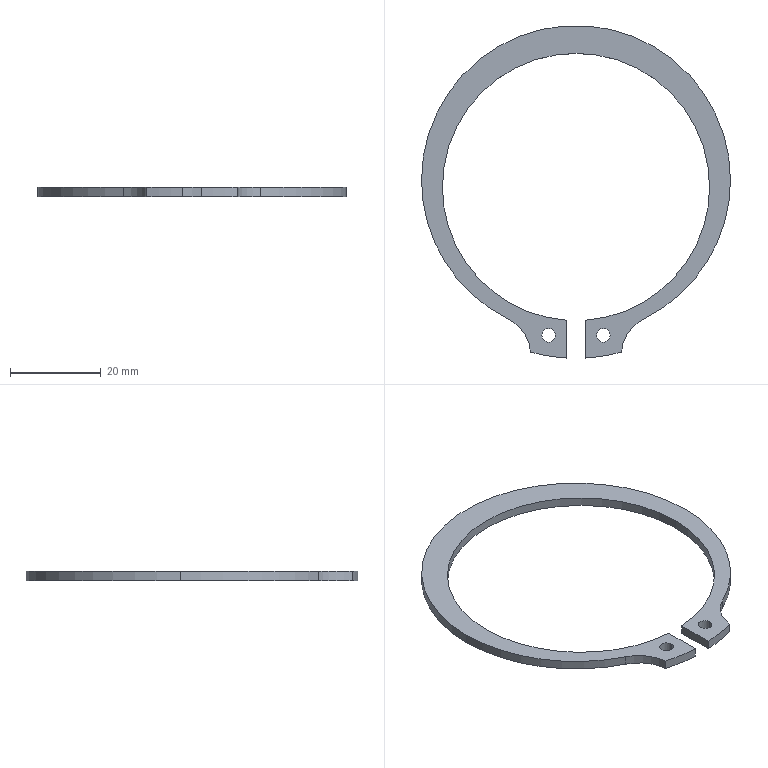Part | STEP file | circlips for shaft--type b gb_GB_CONNECTING_PIECE_RINGS_CSB 63 | 1 solid | 18 faces | box 68 x 73.167 x 2 mm | volume 1973 mm3 | cylinder 14 | plane 4 | commonest cylinder face diameters 3 x4 58.8 x3 68 x3 18 x2 75.38 x2
STEP:
#1=CARTESIAN_POINT('',(0.,0.,0.));
#2=DIRECTION('',(0.,0.,1.));
#3=DIRECTION('',(1.,0.,0.));
#4=AXIS2_PLACEMENT_3D('',#1,#2,#3);
#5=CARTESIAN_POINT('',(7.5,-34.183,-2.));
#6=VERTEX_POINT('',#5);
#7=CARTESIAN_POINT('',(7.5,-34.183,0.));
#8=VERTEX_POINT('',#7);
#9=CARTESIAN_POINT('',(7.5,-34.183,-2.));
#10=DIRECTION('',(0.,0.,1.));
#11=VECTOR('',#10,1.);
#12=LINE('',#9,#11);
#13=CARTESIAN_POINT('',(6.,-34.183,-2.));
#14=DIRECTION('',(0.,0.,1.));
#15=DIRECTION('',(1.,0.,0.));
#16=AXIS2_PLACEMENT_3D('',#13,#14,#15);
#17=CYLINDRICAL_SURFACE('',#16,1.5);
#18=CARTESIAN_POINT('',(6.283,0.));
#19=DIRECTION('',(0.,1.));
#20=VECTOR('',#19,1.);
#21=LINE('',#18,#20);
#22=(GEOMETRIC_REPRESENTATION_CONTEXT(2)PARAMETRIC_REPRESENTATION_CONTEXT()REPRESENTATION_CONTEXT('',''));
#23=DEFINITIONAL_REPRESENTATION('',(#21),#22);
#24=PCURVE('',#17,#23);
#25=CARTESIAN_POINT('',(6.,-34.183,-2.));
#26=DIRECTION('',(0.,0.,1.));
#27=DIRECTION('',(1.,0.,0.));
#28=AXIS2_PLACEMENT_3D('',#25,#26,#27);
#29=CYLINDRICAL_SURFACE('',#28,1.5);
#30=CARTESIAN_POINT('',(0.,0.));
#31=DIRECTION('',(0.,1.));
#32=VECTOR('',#31,1.);
#33=LINE('',#30,#32);
#34=(GEOMETRIC_REPRESENTATION_CONTEXT(2)PARAMETRIC_REPRESENTATION_CONTEXT()REPRESENTATION_CONTEXT('',''));
#35=DEFINITIONAL_REPRESENTATION('',(#33),#34);
#36=PCURVE('',#29,#35);
#37=SURFACE_CURVE('',#12,(#24,#36),.PCURVE_S1.);
#38=EDGE_CURVE('',#6,#8,#37,.T.);
#39=ORIENTED_EDGE('',*,*,#38,.T.);
#40=CARTESIAN_POINT('',(4.5,-34.183,0.));
#41=VERTEX_POINT('',#40);
#42=CARTESIAN_POINT('',(6.,-34.183,0.));
#43=DIRECTION('',(0.,0.,1.));
#44=DIRECTION('',(-1.,0.,0.));
#45=AXIS2_PLACEMENT_3D('',#42,#43,#44);
#46=CIRCLE('',#45,1.5);
#47=CARTESIAN_POINT('',(3.142,2.));
#48=DIRECTION('',(1.,0.));
#49=VECTOR('',#48,1.);
#50=LINE('',#47,#49);
#51=(GEOMETRIC_REPRESENTATION_CONTEXT(2)PARAMETRIC_REPRESENTATION_CONTEXT()REPRESENTATION_CONTEXT('',''));
#52=DEFINITIONAL_REPRESENTATION('',(#50),#51);
#53=PCURVE('',#17,#52);
#54=CARTESIAN_POINT('',(0.,0.,0.));
#55=DIRECTION('',(0.,0.,1.));
#56=DIRECTION('',(1.,0.,0.));
#57=AXIS2_PLACEMENT_3D('',#54,#55,#56);
#58=PLANE('',#57);
#59=CARTESIAN_POINT('',(6.,-34.183));
#60=DIRECTION('',(-1.,0.));
#61=AXIS2_PLACEMENT_2D('',#59,#60);
#62=CIRCLE('',#61,1.5);
#63=(GEOMETRIC_REPRESENTATION_CONTEXT(2)PARAMETRIC_REPRESENTATION_CONTEXT()REPRESENTATION_CONTEXT('',''));
#64=DEFINITIONAL_REPRESENTATION('',(#62),#63);
#65=PCURVE('',#58,#64);
#66=SURFACE_CURVE('',#46,(#53,#65),.PCURVE_S1.);
#67=EDGE_CURVE('',#41,#8,#66,.T.);
#68=ORIENTED_EDGE('',*,*,#67,.F.);
#69=CARTESIAN_POINT('',(4.5,-34.183,-2.));
#70=VERTEX_POINT('',#69);
#71=CARTESIAN_POINT('',(4.5,-34.183,-2.));
#72=DIRECTION('',(0.,0.,1.));
#73=VECTOR('',#72,1.);
#74=LINE('',#71,#73);
#75=CARTESIAN_POINT('',(3.142,0.));
#76=DIRECTION('',(0.,1.));
#77=VECTOR('',#76,1.);
#78=LINE('',#75,#77);
#79=(GEOMETRIC_REPRESENTATION_CONTEXT(2)PARAMETRIC_REPRESENTATION_CONTEXT()REPRESENTATION_CONTEXT('',''));
#80=DEFINITIONAL_REPRESENTATION('',(#78),#79);
#81=PCURVE('',#17,#80);
#82=CARTESIAN_POINT('',(3.142,0.));
#83=DIRECTION('',(0.,1.));
#84=VECTOR('',#83,1.);
#85=LINE('',#82,#84);
#86=(GEOMETRIC_REPRESENTATION_CONTEXT(2)PARAMETRIC_REPRESENTATION_CONTEXT()REPRESENTATION_CONTEXT('',''));
#87=DEFINITIONAL_REPRESENTATION('',(#85),#86);
#88=PCURVE('',#29,#87);
#89=SURFACE_CURVE('',#74,(#81,#88),.PCURVE_S1.);
#90=EDGE_CURVE('',#70,#41,#89,.T.);
#91=ORIENTED_EDGE('',*,*,#90,.F.);
#92=CARTESIAN_POINT('',(6.,-34.183,-2.));
#93=DIRECTION('',(0.,0.,1.));
#94=DIRECTION('',(-1.,0.,0.));
#95=AXIS2_PLACEMENT_3D('',#92,#93,#94);
#96=CIRCLE('',#95,1.5);
#97=CARTESIAN_POINT('',(3.142,0.));
#98=DIRECTION('',(1.,0.));
#99=VECTOR('',#98,1.);
#100=LINE('',#97,#99);
#101=(GEOMETRIC_REPRESENTATION_CONTEXT(2)PARAMETRIC_REPRESENTATION_CONTEXT()REPRESENTATION_CONTEXT('',''));
#102=DEFINITIONAL_REPRESENTATION('',(#100),#101);
#103=PCURVE('',#17,#102);
#104=CARTESIAN_POINT('',(0.,0.,-2.));
#105=DIRECTION('',(0.,0.,1.));
#106=DIRECTION('',(1.,0.,0.));
#107=AXIS2_PLACEMENT_3D('',#104,#105,#106);
#108=PLANE('',#107);
#109=CARTESIAN_POINT('',(6.,-34.183));
#110=DIRECTION('',(-1.,0.));
#111=AXIS2_PLACEMENT_2D('',#109,#110);
#112=CIRCLE('',#111,1.5);
#113=(GEOMETRIC_REPRESENTATION_CONTEXT(2)PARAMETRIC_REPRESENTATION_CONTEXT()REPRESENTATION_CONTEXT('',''));
#114=DEFINITIONAL_REPRESENTATION('',(#112),#113);
#115=PCURVE('',#108,#114);
#116=SURFACE_CURVE('',#96,(#103,#115),.PCURVE_S1.);
#117=EDGE_CURVE('',#70,#6,#116,.T.);
#118=ORIENTED_EDGE('',*,*,#117,.T.);
#119=EDGE_LOOP('',(#39,#68,#91,#118));
#120=FACE_BOUND('',#119,.F.);
#121=ADVANCED_FACE('',(#120),#17,.F.);
#122=CARTESIAN_POINT('',(-4.5,-34.183,-2.));
#123=VERTEX_POINT('',#122);
#124=CARTESIAN_POINT('',(-4.5,-34.183,0.));
#125=VERTEX_POINT('',#124);
#126=CARTESIAN_POINT('',(-4.5,-34.183,-2.));
#127=DIRECTION('',(0.,0.,1.));
#128=VECTOR('',#127,1.);
#129=LINE('',#126,#128);
#130=CARTESIAN_POINT('',(-6.,-34.183,-2.));
#131=DIRECTION('',(0.,0.,1.));
#132=DIRECTION('',(1.,0.,0.));
#133=AXIS2_PLACEMENT_3D('',#130,#131,#132);
#134=CYLINDRICAL_SURFACE('',#133,1.5);
#135=CARTESIAN_POINT('',(6.283,0.));
#136=DIRECTION('',(0.,1.));
#137=VECTOR('',#136,1.);
#138=LINE('',#135,#137);
#139=(GEOMETRIC_REPRESENTATION_CONTEXT(2)PARAMETRIC_REPRESENTATION_CONTEXT()REPRESENTATION_CONTEXT('',''));
#140=DEFINITIONAL_REPRESENTATION('',(#138),#139);
#141=PCURVE('',#134,#140);
#142=CARTESIAN_POINT('',(-6.,-34.183,-2.));
#143=DIRECTION('',(0.,0.,1.));
#144=DIRECTION('',(1.,0.,0.));
#145=AXIS2_PLACEMENT_3D('',#142,#143,#144);
#146=CYLINDRICAL_SURFACE('',#145,1.5);
#147=CARTESIAN_POINT('',(0.,0.));
#148=DIRECTION('',(0.,1.));
#149=VECTOR('',#148,1.);
#150=LINE('',#147,#149);
#151=(GEOMETRIC_REPRESENTATION_CONTEXT(2)PARAMETRIC_REPRESENTATION_CONTEXT()REPRESENTATION_CONTEXT('',''));
#152=DEFINITIONAL_REPRESENTATION('',(#150),#151);
#153=PCURVE('',#146,#152);
#154=SURFACE_CURVE('',#129,(#141,#153),.PCURVE_S1.);
#155=EDGE_CURVE('',#123,#125,#154,.T.);
#156=ORIENTED_EDGE('',*,*,#155,.T.);
#157=CARTESIAN_POINT('',(-7.5,-34.183,0.));
#158=VERTEX_POINT('',#157);
#159=CARTESIAN_POINT('',(-6.,-34.183,0.));
#160=DIRECTION('',(0.,0.,1.));
#161=DIRECTION('',(1.,0.,0.));
#162=AXIS2_PLACEMENT_3D('',#159,#160,#161);
#163=CIRCLE('',#162,1.5);
#164=CARTESIAN_POINT('',(0.,2.));
#165=DIRECTION('',(1.,0.));
#166=VECTOR('',#165,1.);
#167=LINE('',#164,#166);
#168=(GEOMETRIC_REPRESENTATION_CONTEXT(2)PARAMETRIC_REPRESENTATION_CONTEXT()REPRESENTATION_CONTEXT('',''));
#169=DEFINITIONAL_REPRESENTATION('',(#167),#168);
#170=PCURVE('',#134,#169);
#171=CARTESIAN_POINT('',(-6.,-34.183));
#172=DIRECTION('',(1.,0.));
#173=AXIS2_PLACEMENT_2D('',#171,#172);
#174=CIRCLE('',#173,1.5);
#175=(GEOMETRIC_REPRESENTATION_CONTEXT(2)PARAMETRIC_REPRESENTATION_CONTEXT()REPRESENTATION_CONTEXT('',''));
#176=DEFINITIONAL_REPRESENTATION('',(#174),#175);
#177=PCURVE('',#58,#176);
#178=SURFACE_CURVE('',#163,(#170,#177),.PCURVE_S1.);
#179=EDGE_CURVE('',#158,#125,#178,.T.);
#180=ORIENTED_EDGE('',*,*,#179,.F.);
#181=CARTESIAN_POINT('',(-7.5,-34.183,-2.));
#182=VERTEX_POINT('',#181);
#183=CARTESIAN_POINT('',(-7.5,-34.183,-2.));
#184=DIRECTION('',(0.,0.,1.));
#185=VECTOR('',#184,1.);
#186=LINE('',#183,#185);
#187=CARTESIAN_POINT('',(3.142,0.));
#188=DIRECTION('',(0.,1.));
#189=VECTOR('',#188,1.);
#190=LINE('',#187,#189);
#191=(GEOMETRIC_REPRESENTATION_CONTEXT(2)PARAMETRIC_REPRESENTATION_CONTEXT()REPRESENTATION_CONTEXT('',''));
#192=DEFINITIONAL_REPRESENTATION('',(#190),#191);
#193=PCURVE('',#134,#192);
#194=CARTESIAN_POINT('',(3.142,0.));
#195=DIRECTION('',(0.,1.));
#196=VECTOR('',#195,1.);
#197=LINE('',#194,#196);
#198=(GEOMETRIC_REPRESENTATION_CONTEXT(2)PARAMETRIC_REPRESENTATION_CONTEXT()REPRESENTATION_CONTEXT('',''));
#199=DEFINITIONAL_REPRESENTATION('',(#197),#198);
#200=PCURVE('',#146,#199);
#201=SURFACE_CURVE('',#186,(#193,#200),.PCURVE_S1.);
#202=EDGE_CURVE('',#182,#158,#201,.T.);
#203=ORIENTED_EDGE('',*,*,#202,.F.);
#204=CARTESIAN_POINT('',(-6.,-34.183,-2.));
#205=DIRECTION('',(0.,0.,1.));
#206=DIRECTION('',(1.,0.,0.));
#207=AXIS2_PLACEMENT_3D('',#204,#205,#206);
#208=CIRCLE('',#207,1.5);
#209=CARTESIAN_POINT('',(0.,0.));
#210=DIRECTION('',(1.,0.));
#211=VECTOR('',#210,1.);
#212=LINE('',#209,#211);
#213=(GEOMETRIC_REPRESENTATION_CONTEXT(2)PARAMETRIC_REPRESENTATION_CONTEXT()REPRESENTATION_CONTEXT('',''));
#214=DEFINITIONAL_REPRESENTATION('',(#212),#213);
#215=PCURVE('',#134,#214);
#216=CARTESIAN_POINT('',(-6.,-34.183));
#217=DIRECTION('',(1.,0.));
#218=AXIS2_PLACEMENT_2D('',#216,#217);
#219=CIRCLE('',#218,1.5);
#220=(GEOMETRIC_REPRESENTATION_CONTEXT(2)PARAMETRIC_REPRESENTATION_CONTEXT()REPRESENTATION_CONTEXT('',''));
#221=DEFINITIONAL_REPRESENTATION('',(#219),#220);
#222=PCURVE('',#108,#221);
#223=SURFACE_CURVE('',#208,(#215,#222),.PCURVE_S1.);
#224=EDGE_CURVE('',#182,#123,#223,.T.);
#225=ORIENTED_EDGE('',*,*,#224,.T.);
#226=EDGE_LOOP('',(#156,#180,#203,#225));
#227=FACE_BOUND('',#226,.F.);
#228=ADVANCED_FACE('',(#227),#134,.F.);
#229=CARTESIAN_POINT('',(-2.,-30.862,-2.));
#230=VERTEX_POINT('',#229);
#231=CARTESIAN_POINT('',(-2.,-30.862,0.));
#232=VERTEX_POINT('',#231);
#233=CARTESIAN_POINT('',(-2.,-30.862,-2.));
#234=DIRECTION('',(0.,0.,1.));
#235=VECTOR('',#234,1.);
#236=LINE('',#233,#235);
#237=CARTESIAN_POINT('',(0.,-1.53,-2.));
#238=DIRECTION('',(0.,0.,1.));
#239=DIRECTION('',(1.,0.,0.));
#240=AXIS2_PLACEMENT_3D('',#237,#238,#239);
#241=CYLINDRICAL_SURFACE('',#240,29.4);
#242=CARTESIAN_POINT('',(4.644,0.));
#243=DIRECTION('',(0.,1.));
#244=VECTOR('',#243,1.);
#245=LINE('',#242,#244);
#246=(GEOMETRIC_REPRESENTATION_CONTEXT(2)PARAMETRIC_REPRESENTATION_CONTEXT()REPRESENTATION_CONTEXT('',''));
#247=DEFINITIONAL_REPRESENTATION('',(#245),#246);
#248=PCURVE('',#241,#247);
#249=CARTESIAN_POINT('',(-2.,-39.167,-2.));
#250=DIRECTION('',(1.,0.,0.));
#251=DIRECTION('',(0.,1.,0.));
#252=AXIS2_PLACEMENT_3D('',#249,#250,#251);
#253=PLANE('',#252);
#254=CARTESIAN_POINT('',(8.305,0.));
#255=DIRECTION('',(0.,1.));
#256=VECTOR('',#255,1.);
#257=LINE('',#254,#256);
#258=(GEOMETRIC_REPRESENTATION_CONTEXT(2)PARAMETRIC_REPRESENTATION_CONTEXT()REPRESENTATION_CONTEXT('',''));
#259=DEFINITIONAL_REPRESENTATION('',(#257),#258);
#260=PCURVE('',#253,#259);
#261=SURFACE_CURVE('',#236,(#248,#260),.PCURVE_S1.);
#262=EDGE_CURVE('',#230,#232,#261,.T.);
#263=ORIENTED_EDGE('',*,*,#262,.T.);
#264=CARTESIAN_POINT('',(-29.4,-1.53,0.));
#265=VERTEX_POINT('',#264);
#266=CARTESIAN_POINT('',(0.,-1.53,0.));
#267=DIRECTION('',(0.,0.,-1.));
#268=DIRECTION('',(1.,0.,0.));
#269=AXIS2_PLACEMENT_3D('',#266,#267,#268);
#270=CIRCLE('',#269,29.4);
#271=CARTESIAN_POINT('',(6.283,2.));
#272=DIRECTION('',(-1.,0.));
#273=VECTOR('',#272,1.);
#274=LINE('',#271,#273);
#275=(GEOMETRIC_REPRESENTATION_CONTEXT(2)PARAMETRIC_REPRESENTATION_CONTEXT()REPRESENTATION_CONTEXT('',''));
#276=DEFINITIONAL_REPRESENTATION('',(#274),#275);
#277=PCURVE('',#241,#276);
#278=CARTESIAN_POINT('',(29.4,-1.53));
#279=CARTESIAN_POINT('',(29.4,-52.452));
#280=CARTESIAN_POINT('',(-14.7,-26.991));
#281=CARTESIAN_POINT('',(-58.8,-1.53));
#282=CARTESIAN_POINT('',(-14.7,23.931));
#283=CARTESIAN_POINT('',(29.4,49.392));
#284=CARTESIAN_POINT('',(29.4,-1.53));
#285=(BOUNDED_CURVE()B_SPLINE_CURVE(2,(#278,#279,#280,#281,#282,#283,#284),.UNSPECIFIED.,.T.,.F.)B_SPLINE_CURVE_WITH_KNOTS((1,2,2,2,2,1),(-2.094,0.,2.094,4.189,6.283,8.378),.UNSPECIFIED.)CURVE()GEOMETRIC_REPRESENTATION_ITEM()RATIONAL_B_SPLINE_CURVE((1.,0.5,1.,0.5,1.,0.5,1.))REPRESENTATION_ITEM(''));
#286=(GEOMETRIC_REPRESENTATION_CONTEXT(2)PARAMETRIC_REPRESENTATION_CONTEXT()REPRESENTATION_CONTEXT('',''));
#287=DEFINITIONAL_REPRESENTATION('',(#285),#286);
#288=PCURVE('',#58,#287);
#289=SURFACE_CURVE('',#270,(#277,#288),.PCURVE_S1.);
#290=EDGE_CURVE('',#232,#265,#289,.T.);
#291=ORIENTED_EDGE('',*,*,#290,.T.);
#292=CARTESIAN_POINT('',(-29.4,-1.53,-2.));
#293=VERTEX_POINT('',#292);
#294=CARTESIAN_POINT('',(-29.4,-1.53,-2.));
#295=DIRECTION('',(0.,0.,1.));
#296=VECTOR('',#295,1.);
#297=LINE('',#294,#296);
#298=CARTESIAN_POINT('',(3.142,0.));
#299=DIRECTION('',(0.,1.));
#300=VECTOR('',#299,1.);
#301=LINE('',#298,#300);
#302=(GEOMETRIC_REPRESENTATION_CONTEXT(2)PARAMETRIC_REPRESENTATION_CONTEXT()REPRESENTATION_CONTEXT('',''));
#303=DEFINITIONAL_REPRESENTATION('',(#301),#302);
#304=PCURVE('',#241,#303);
#305=CARTESIAN_POINT('',(0.,-1.53,-2.));
#306=DIRECTION('',(0.,0.,1.));
#307=DIRECTION('',(1.,0.,0.));
#308=AXIS2_PLACEMENT_3D('',#305,#306,#307);
#309=CYLINDRICAL_SURFACE('',#308,29.4);
#310=CARTESIAN_POINT('',(3.142,0.));
#311=DIRECTION('',(0.,1.));
#312=VECTOR('',#311,1.);
#313=LINE('',#310,#312);
#314=(GEOMETRIC_REPRESENTATION_CONTEXT(2)PARAMETRIC_REPRESENTATION_CONTEXT()REPRESENTATION_CONTEXT('',''));
#315=DEFINITIONAL_REPRESENTATION('',(#313),#314);
#316=PCURVE('',#309,#315);
#317=SURFACE_CURVE('',#297,(#304,#316),.PCURVE_S1.);
#318=EDGE_CURVE('',#293,#265,#317,.T.);
#319=ORIENTED_EDGE('',*,*,#318,.F.);
#320=CARTESIAN_POINT('',(0.,-1.53,-2.));
#321=DIRECTION('',(0.,0.,-1.));
#322=DIRECTION('',(1.,0.,0.));
#323=AXIS2_PLACEMENT_3D('',#320,#321,#322);
#324=CIRCLE('',#323,29.4);
#325=CARTESIAN_POINT('',(6.283,0.));
#326=DIRECTION('',(-1.,0.));
#327=VECTOR('',#326,1.);
#328=LINE('',#325,#327);
#329=(GEOMETRIC_REPRESENTATION_CONTEXT(2)PARAMETRIC_REPRESENTATION_CONTEXT()REPRESENTATION_CONTEXT('',''));
#330=DEFINITIONAL_REPRESENTATION('',(#328),#329);
#331=PCURVE('',#241,#330);
#332=CARTESIAN_POINT('',(29.4,-1.53));
#333=CARTESIAN_POINT('',(29.4,-52.452));
#334=CARTESIAN_POINT('',(-14.7,-26.991));
#335=CARTESIAN_POINT('',(-58.8,-1.53));
#336=CARTESIAN_POINT('',(-14.7,23.931));
#337=CARTESIAN_POINT('',(29.4,49.392));
#338=CARTESIAN_POINT('',(29.4,-1.53));
#339=(BOUNDED_CURVE()B_SPLINE_CURVE(2,(#332,#333,#334,#335,#336,#337,#338),.UNSPECIFIED.,.T.,.F.)B_SPLINE_CURVE_WITH_KNOTS((1,2,2,2,2,1),(-2.094,0.,2.094,4.189,6.283,8.378),.UNSPECIFIED.)CURVE()GEOMETRIC_REPRESENTATION_ITEM()RATIONAL_B_SPLINE_CURVE((1.,0.5,1.,0.5,1.,0.5,1.))REPRESENTATION_ITEM(''));
#340=(GEOMETRIC_REPRESENTATION_CONTEXT(2)PARAMETRIC_REPRESENTATION_CONTEXT()REPRESENTATION_CONTEXT('',''));
#341=DEFINITIONAL_REPRESENTATION('',(#339),#340);
#342=PCURVE('',#108,#341);
#343=SURFACE_CURVE('',#324,(#331,#342),.PCURVE_S1.);
#344=EDGE_CURVE('',#230,#293,#343,.T.);
#345=ORIENTED_EDGE('',*,*,#344,.F.);
#346=EDGE_LOOP('',(#263,#291,#319,#345));
#347=FACE_BOUND('',#346,.F.);
#348=ADVANCED_FACE('',(#347),#241,.F.);
#349=CARTESIAN_POINT('',(29.4,-1.53,0.));
#350=VERTEX_POINT('',#349);
#351=CARTESIAN_POINT('',(0.,-1.53,0.));
#352=DIRECTION('',(0.,0.,-1.));
#353=DIRECTION('',(1.,0.,0.));
#354=AXIS2_PLACEMENT_3D('',#351,#352,#353);
#355=CIRCLE('',#354,29.4);
#356=CARTESIAN_POINT('',(6.283,2.));
#357=DIRECTION('',(-1.,0.));
#358=VECTOR('',#357,1.);
#359=LINE('',#356,#358);
#360=(GEOMETRIC_REPRESENTATION_CONTEXT(2)PARAMETRIC_REPRESENTATION_CONTEXT()REPRESENTATION_CONTEXT('',''));
#361=DEFINITIONAL_REPRESENTATION('',(#359),#360);
#362=PCURVE('',#309,#361);
#363=CARTESIAN_POINT('',(29.4,-1.53));
#364=CARTESIAN_POINT('',(29.4,-52.452));
#365=CARTESIAN_POINT('',(-14.7,-26.991));
#366=CARTESIAN_POINT('',(-58.8,-1.53));
#367=CARTESIAN_POINT('',(-14.7,23.931));
#368=CARTESIAN_POINT('',(29.4,49.392));
#369=CARTESIAN_POINT('',(29.4,-1.53));
#370=(BOUNDED_CURVE()B_SPLINE_CURVE(2,(#363,#364,#365,#366,#367,#368,#369),.UNSPECIFIED.,.T.,.F.)B_SPLINE_CURVE_WITH_KNOTS((1,2,2,2,2,1),(-2.094,0.,2.094,4.189,6.283,8.378),.UNSPECIFIED.)CURVE()GEOMETRIC_REPRESENTATION_ITEM()RATIONAL_B_SPLINE_CURVE((1.,0.5,1.,0.5,1.,0.5,1.))REPRESENTATION_ITEM(''));
#371=(GEOMETRIC_REPRESENTATION_CONTEXT(2)PARAMETRIC_REPRESENTATION_CONTEXT()REPRESENTATION_CONTEXT('',''));
#372=DEFINITIONAL_REPRESENTATION('',(#370),#371);
#373=PCURVE('',#58,#372);
#374=SURFACE_CURVE('',#355,(#362,#373),.PCURVE_S1.);
#375=EDGE_CURVE('',#265,#350,#374,.T.);
#376=ORIENTED_EDGE('',*,*,#375,.T.);
#377=CARTESIAN_POINT('',(29.4,-1.53,-2.));
#378=VERTEX_POINT('',#377);
#379=CARTESIAN_POINT('',(29.4,-1.53,-2.));
#380=DIRECTION('',(0.,0.,1.));
#381=VECTOR('',#380,1.);
#382=LINE('',#379,#381);
#383=CARTESIAN_POINT('',(0.,0.));
#384=DIRECTION('',(0.,1.));
#385=VECTOR('',#384,1.);
#386=LINE('',#383,#385);
#387=(GEOMETRIC_REPRESENTATION_CONTEXT(2)PARAMETRIC_REPRESENTATION_CONTEXT()REPRESENTATION_CONTEXT('',''));
#388=DEFINITIONAL_REPRESENTATION('',(#386),#387);
#389=PCURVE('',#309,#388);
#390=CARTESIAN_POINT('',(0.,-1.53,-2.));
#391=DIRECTION('',(0.,0.,1.));
#392=DIRECTION('',(1.,0.,0.));
#393=AXIS2_PLACEMENT_3D('',#390,#391,#392);
#394=CYLINDRICAL_SURFACE('',#393,29.4);
#395=CARTESIAN_POINT('',(6.283,0.));
#396=DIRECTION('',(0.,1.));
#397=VECTOR('',#396,1.);
#398=LINE('',#395,#397);
#399=(GEOMETRIC_REPRESENTATION_CONTEXT(2)PARAMETRIC_REPRESENTATION_CONTEXT()REPRESENTATION_CONTEXT('',''));
#400=DEFINITIONAL_REPRESENTATION('',(#398),#399);
#401=PCURVE('',#394,#400);
#402=SURFACE_CURVE('',#382,(#389,#401),.PCURVE_S1.);
#403=EDGE_CURVE('',#378,#350,#402,.T.);
#404=ORIENTED_EDGE('',*,*,#403,.F.);
#405=CARTESIAN_POINT('',(0.,-1.53,-2.));
#406=DIRECTION('',(0.,0.,-1.));
#407=DIRECTION('',(1.,0.,0.));
#408=AXIS2_PLACEMENT_3D('',#405,#406,#407);
#409=CIRCLE('',#408,29.4);
#410=CARTESIAN_POINT('',(6.283,0.));
#411=DIRECTION('',(-1.,0.));
#412=VECTOR('',#411,1.);
#413=LINE('',#410,#412);
#414=(GEOMETRIC_REPRESENTATION_CONTEXT(2)PARAMETRIC_REPRESENTATION_CONTEXT()REPRESENTATION_CONTEXT('',''));
#415=DEFINITIONAL_REPRESENTATION('',(#413),#414);
#416=PCURVE('',#309,#415);
#417=CARTESIAN_POINT('',(29.4,-1.53));
#418=CARTESIAN_POINT('',(29.4,-52.452));
#419=CARTESIAN_POINT('',(-14.7,-26.991));
#420=CARTESIAN_POINT('',(-58.8,-1.53));
#421=CARTESIAN_POINT('',(-14.7,23.931));
#422=CARTESIAN_POINT('',(29.4,49.392));
#423=CARTESIAN_POINT('',(29.4,-1.53));
#424=(BOUNDED_CURVE()B_SPLINE_CURVE(2,(#417,#418,#419,#420,#421,#422,#423),.UNSPECIFIED.,.T.,.F.)B_SPLINE_CURVE_WITH_KNOTS((1,2,2,2,2,1),(-2.094,0.,2.094,4.189,6.283,8.378),.UNSPECIFIED.)CURVE()GEOMETRIC_REPRESENTATION_ITEM()RATIONAL_B_SPLINE_CURVE((1.,0.5,1.,0.5,1.,0.5,1.))REPRESENTATION_ITEM(''));
#425=(GEOMETRIC_REPRESENTATION_CONTEXT(2)PARAMETRIC_REPRESENTATION_CONTEXT()REPRESENTATION_CONTEXT('',''));
#426=DEFINITIONAL_REPRESENTATION('',(#424),#425);
#427=PCURVE('',#108,#426);
#428=SURFACE_CURVE('',#409,(#416,#427),.PCURVE_S1.);
#429=EDGE_CURVE('',#293,#378,#428,.T.);
#430=ORIENTED_EDGE('',*,*,#429,.F.);
#431=ORIENTED_EDGE('',*,*,#318,.T.);
#432=EDGE_LOOP('',(#376,#404,#430,#431));
#433=FACE_BOUND('',#432,.F.);
#434=ADVANCED_FACE('',(#433),#309,.F.);
#435=CARTESIAN_POINT('',(34.,0.,-2.));
#436=VERTEX_POINT('',#435);
#437=CARTESIAN_POINT('',(-34.,0.,-2.));
#438=VERTEX_POINT('',#437);
#439=CARTESIAN_POINT('',(0.,0.,-2.));
#440=DIRECTION('',(0.,0.,1.));
#441=DIRECTION('',(1.,0.,0.));
#442=AXIS2_PLACEMENT_3D('',#439,#440,#441);
#443=CIRCLE('',#442,34.);
#444=CARTESIAN_POINT('',(0.,0.,-2.));
#445=DIRECTION('',(0.,0.,1.));
#446=DIRECTION('',(1.,0.,0.));
#447=AXIS2_PLACEMENT_3D('',#444,#445,#446);
#448=CYLINDRICAL_SURFACE('',#447,34.);
#449=CARTESIAN_POINT('',(0.,0.));
#450=DIRECTION('',(1.,0.));
#451=VECTOR('',#450,1.);
#452=LINE('',#449,#451);
#453=(GEOMETRIC_REPRESENTATION_CONTEXT(2)PARAMETRIC_REPRESENTATION_CONTEXT()REPRESENTATION_CONTEXT('',''));
#454=DEFINITIONAL_REPRESENTATION('',(#452),#453);
#455=PCURVE('',#448,#454);
#456=CARTESIAN_POINT('',(0.,0.));
#457=DIRECTION('',(1.,0.));
#458=AXIS2_PLACEMENT_2D('',#456,#457);
#459=CIRCLE('',#458,34.);
#460=(GEOMETRIC_REPRESENTATION_CONTEXT(2)PARAMETRIC_REPRESENTATION_CONTEXT()REPRESENTATION_CONTEXT('',''));
#461=DEFINITIONAL_REPRESENTATION('',(#459),#460);
#462=PCURVE('',#108,#461);
#463=SURFACE_CURVE('',#443,(#455,#462),.PCURVE_S1.);
#464=EDGE_CURVE('',#436,#438,#463,.T.);
#465=ORIENTED_EDGE('',*,*,#464,.T.);
#466=CARTESIAN_POINT('',(-34.,0.,0.));
#467=VERTEX_POINT('',#466);
#468=CARTESIAN_POINT('',(-34.,0.,-2.));
#469=DIRECTION('',(0.,0.,1.));
#470=VECTOR('',#469,1.);
#471=LINE('',#468,#470);
#472=CARTESIAN_POINT('',(3.142,0.));
#473=DIRECTION('',(0.,1.));
#474=VECTOR('',#473,1.);
#475=LINE('',#472,#474);
#476=(GEOMETRIC_REPRESENTATION_CONTEXT(2)PARAMETRIC_REPRESENTATION_CONTEXT()REPRESENTATION_CONTEXT('',''));
#477=DEFINITIONAL_REPRESENTATION('',(#475),#476);
#478=PCURVE('',#448,#477);
#479=CARTESIAN_POINT('',(0.,0.,-2.));
#480=DIRECTION('',(0.,0.,1.));
#481=DIRECTION('',(1.,0.,0.));
#482=AXIS2_PLACEMENT_3D('',#479,#480,#481);
#483=CYLINDRICAL_SURFACE('',#482,34.);
#484=CARTESIAN_POINT('',(3.142,0.));
#485=DIRECTION('',(0.,1.));
#486=VECTOR('',#485,1.);
#487=LINE('',#484,#486);
#488=(GEOMETRIC_REPRESENTATION_CONTEXT(2)PARAMETRIC_REPRESENTATION_CONTEXT()REPRESENTATION_CONTEXT('',''));
#489=DEFINITIONAL_REPRESENTATION('',(#487),#488);
#490=PCURVE('',#483,#489);
#491=SURFACE_CURVE('',#471,(#478,#490),.PCURVE_S1.);
#492=EDGE_CURVE('',#438,#467,#491,.T.);
#493=ORIENTED_EDGE('',*,*,#492,.T.);
#494=CARTESIAN_POINT('',(34.,0.,0.));
#495=VERTEX_POINT('',#494);
#496=CARTESIAN_POINT('',(0.,0.,0.));
#497=DIRECTION('',(0.,0.,1.));
#498=DIRECTION('',(1.,0.,0.));
#499=AXIS2_PLACEMENT_3D('',#496,#497,#498);
#500=CIRCLE('',#499,34.);
#501=CARTESIAN_POINT('',(0.,2.));
#502=DIRECTION('',(1.,0.));
#503=VECTOR('',#502,1.);
#504=LINE('',#501,#503);
#505=(GEOMETRIC_REPRESENTATION_CONTEXT(2)PARAMETRIC_REPRESENTATION_CONTEXT()REPRESENTATION_CONTEXT('',''));
#506=DEFINITIONAL_REPRESENTATION('',(#504),#505);
#507=PCURVE('',#448,#506);
#508=CARTESIAN_POINT('',(0.,0.));
#509=DIRECTION('',(1.,0.));
#510=AXIS2_PLACEMENT_2D('',#508,#509);
#511=CIRCLE('',#510,34.);
#512=(GEOMETRIC_REPRESENTATION_CONTEXT(2)PARAMETRIC_REPRESENTATION_CONTEXT()REPRESENTATION_CONTEXT('',''));
#513=DEFINITIONAL_REPRESENTATION('',(#511),#512);
#514=PCURVE('',#58,#513);
#515=SURFACE_CURVE('',#500,(#507,#514),.PCURVE_S1.);
#516=EDGE_CURVE('',#495,#467,#515,.T.);
#517=ORIENTED_EDGE('',*,*,#516,.F.);
#518=CARTESIAN_POINT('',(34.,0.,-2.));
#519=DIRECTION('',(0.,0.,1.));
#520=VECTOR('',#519,1.);
#521=LINE('',#518,#520);
#522=CARTESIAN_POINT('',(0.,0.));
#523=DIRECTION('',(0.,1.));
#524=VECTOR('',#523,1.);
#525=LINE('',#522,#524);
#526=(GEOMETRIC_REPRESENTATION_CONTEXT(2)PARAMETRIC_REPRESENTATION_CONTEXT()REPRESENTATION_CONTEXT('',''));
#527=DEFINITIONAL_REPRESENTATION('',(#525),#526);
#528=PCURVE('',#448,#527);
#529=CARTESIAN_POINT('',(0.,0.,-2.));
#530=DIRECTION('',(0.,0.,1.));
#531=DIRECTION('',(1.,0.,0.));
#532=AXIS2_PLACEMENT_3D('',#529,#530,#531);
#533=CYLINDRICAL_SURFACE('',#532,34.);
#534=CARTESIAN_POINT('',(6.283,0.));
#535=DIRECTION('',(0.,1.));
#536=VECTOR('',#535,1.);
#537=LINE('',#534,#536);
#538=(GEOMETRIC_REPRESENTATION_CONTEXT(2)PARAMETRIC_REPRESENTATION_CONTEXT()REPRESENTATION_CONTEXT('',''));
#539=DEFINITIONAL_REPRESENTATION('',(#537),#538);
#540=PCURVE('',#533,#539);
#541=SURFACE_CURVE('',#521,(#528,#540),.PCURVE_S1.);
#542=EDGE_CURVE('',#436,#495,#541,.T.);
#543=ORIENTED_EDGE('',*,*,#542,.F.);
#544=EDGE_LOOP('',(#465,#493,#517,#543));
#545=FACE_BOUND('',#544,.T.);
#546=ADVANCED_FACE('',(#545),#448,.T.);
#547=CARTESIAN_POINT('',(15.,-30.512,-2.));
#548=VERTEX_POINT('',#547);
#549=CARTESIAN_POINT('',(0.,0.,-2.));
#550=DIRECTION('',(0.,0.,1.));
#551=DIRECTION('',(1.,0.,0.));
#552=AXIS2_PLACEMENT_3D('',#549,#550,#551);
#553=CIRCLE('',#552,34.);
#554=CARTESIAN_POINT('',(0.,0.));
#555=DIRECTION('',(1.,0.));
#556=VECTOR('',#555,1.);
#557=LINE('',#554,#556);
#558=(GEOMETRIC_REPRESENTATION_CONTEXT(2)PARAMETRIC_REPRESENTATION_CONTEXT()REPRESENTATION_CONTEXT('',''));
#559=DEFINITIONAL_REPRESENTATION('',(#557),#558);
#560=PCURVE('',#533,#559);
#561=CARTESIAN_POINT('',(0.,0.));
#562=DIRECTION('',(1.,0.));
#563=AXIS2_PLACEMENT_2D('',#561,#562);
#564=CIRCLE('',#563,34.);
#565=(GEOMETRIC_REPRESENTATION_CONTEXT(2)PARAMETRIC_REPRESENTATION_CONTEXT()REPRESENTATION_CONTEXT('',''));
#566=DEFINITIONAL_REPRESENTATION('',(#564),#565);
#567=PCURVE('',#108,#566);
#568=SURFACE_CURVE('',#553,(#560,#567),.PCURVE_S1.);
#569=EDGE_CURVE('',#548,#436,#568,.T.);
#570=ORIENTED_EDGE('',*,*,#569,.T.);
#571=ORIENTED_EDGE('',*,*,#542,.T.);
#572=CARTESIAN_POINT('',(15.,-30.512,0.));
#573=VERTEX_POINT('',#572);
#574=CARTESIAN_POINT('',(0.,0.,0.));
#575=DIRECTION('',(0.,0.,1.));
#576=DIRECTION('',(1.,0.,0.));
#577=AXIS2_PLACEMENT_3D('',#574,#575,#576);
#578=CIRCLE('',#577,34.);
#579=CARTESIAN_POINT('',(0.,2.));
#580=DIRECTION('',(1.,0.));
#581=VECTOR('',#580,1.);
#582=LINE('',#579,#581);
#583=(GEOMETRIC_REPRESENTATION_CONTEXT(2)PARAMETRIC_REPRESENTATION_CONTEXT()REPRESENTATION_CONTEXT('',''));
#584=DEFINITIONAL_REPRESENTATION('',(#582),#583);
#585=PCURVE('',#533,#584);
#586=CARTESIAN_POINT('',(0.,0.));
#587=DIRECTION('',(1.,0.));
#588=AXIS2_PLACEMENT_2D('',#586,#587);
#589=CIRCLE('',#588,34.);
#590=(GEOMETRIC_REPRESENTATION_CONTEXT(2)PARAMETRIC_REPRESENTATION_CONTEXT()REPRESENTATION_CONTEXT('',''));
#591=DEFINITIONAL_REPRESENTATION('',(#589),#590);
#592=PCURVE('',#58,#591);
#593=SURFACE_CURVE('',#578,(#585,#592),.PCURVE_S1.);
#594=EDGE_CURVE('',#573,#495,#593,.T.);
#595=ORIENTED_EDGE('',*,*,#594,.F.);
#596=CARTESIAN_POINT('',(15.,-30.512,-2.));
#597=DIRECTION('',(0.,0.,-1.));
#598=VECTOR('',#597,1.);
#599=LINE('',#596,#598);
#600=CARTESIAN_POINT('',(5.169,0.));
#601=DIRECTION('',(0.,-1.));
#602=VECTOR('',#601,1.);
#603=LINE('',#600,#602);
#604=(GEOMETRIC_REPRESENTATION_CONTEXT(2)PARAMETRIC_REPRESENTATION_CONTEXT()REPRESENTATION_CONTEXT('',''));
#605=DEFINITIONAL_REPRESENTATION('',(#603),#604);
#606=PCURVE('',#533,#605);
#607=CARTESIAN_POINT('',(18.971,-38.589,-2.));
#608=DIRECTION('',(0.,0.,-1.));
#609=DIRECTION('',(-1.,0.,0.));
#610=AXIS2_PLACEMENT_3D('',#607,#608,#609);
#611=CYLINDRICAL_SURFACE('',#610,9.);
#612=CARTESIAN_POINT('',(1.114,0.));
#613=DIRECTION('',(0.,1.));
#614=VECTOR('',#613,1.);
#615=LINE('',#612,#614);
#616=(GEOMETRIC_REPRESENTATION_CONTEXT(2)PARAMETRIC_REPRESENTATION_CONTEXT()REPRESENTATION_CONTEXT('',''));
#617=DEFINITIONAL_REPRESENTATION('',(#615),#616);
#618=PCURVE('',#611,#617);
#619=SURFACE_CURVE('',#599,(#606,#618),.PCURVE_S1.);
#620=EDGE_CURVE('',#573,#548,#619,.T.);
#621=ORIENTED_EDGE('',*,*,#620,.T.);
#622=EDGE_LOOP('',(#570,#571,#595,#621));
#623=FACE_BOUND('',#622,.T.);
#624=ADVANCED_FACE('',(#623),#533,.T.);
#625=ORIENTED_EDGE('',*,*,#492,.F.);
#626=CARTESIAN_POINT('',(-15.,-30.512,-2.));
#627=VERTEX_POINT('',#626);
#628=CARTESIAN_POINT('',(0.,0.,-2.));
#629=DIRECTION('',(0.,0.,1.));
#630=DIRECTION('',(1.,0.,0.));
#631=AXIS2_PLACEMENT_3D('',#628,#629,#630);
#632=CIRCLE('',#631,34.);
#633=CARTESIAN_POINT('',(0.,0.));
#634=DIRECTION('',(1.,0.));
#635=VECTOR('',#634,1.);
#636=LINE('',#633,#635);
#637=(GEOMETRIC_REPRESENTATION_CONTEXT(2)PARAMETRIC_REPRESENTATION_CONTEXT()REPRESENTATION_CONTEXT('',''));
#638=DEFINITIONAL_REPRESENTATION('',(#636),#637);
#639=PCURVE('',#483,#638);
#640=CARTESIAN_POINT('',(0.,0.));
#641=DIRECTION('',(1.,0.));
#642=AXIS2_PLACEMENT_2D('',#640,#641);
#643=CIRCLE('',#642,34.);
#644=(GEOMETRIC_REPRESENTATION_CONTEXT(2)PARAMETRIC_REPRESENTATION_CONTEXT()REPRESENTATION_CONTEXT('',''));
#645=DEFINITIONAL_REPRESENTATION('',(#643),#644);
#646=PCURVE('',#108,#645);
#647=SURFACE_CURVE('',#632,(#639,#646),.PCURVE_S1.);
#648=EDGE_CURVE('',#438,#627,#647,.T.);
#649=ORIENTED_EDGE('',*,*,#648,.T.);
#650=CARTESIAN_POINT('',(-15.,-30.512,0.));
#651=VERTEX_POINT('',#650);
#652=CARTESIAN_POINT('',(-15.,-30.512,-2.));
#653=DIRECTION('',(0.,0.,1.));
#654=VECTOR('',#653,1.);
#655=LINE('',#652,#654);
#656=CARTESIAN_POINT('',(4.255,0.));
#657=DIRECTION('',(0.,1.));
#658=VECTOR('',#657,1.);
#659=LINE('',#656,#658);
#660=(GEOMETRIC_REPRESENTATION_CONTEXT(2)PARAMETRIC_REPRESENTATION_CONTEXT()REPRESENTATION_CONTEXT('',''));
#661=DEFINITIONAL_REPRESENTATION('',(#659),#660);
#662=PCURVE('',#483,#661);
#663=CARTESIAN_POINT('',(-18.971,-38.589,-2.));
#664=DIRECTION('',(0.,0.,-1.));
#665=DIRECTION('',(-1.,0.,0.));
#666=AXIS2_PLACEMENT_3D('',#663,#664,#665);
#667=CYLINDRICAL_SURFACE('',#666,9.);
#668=CARTESIAN_POINT('',(2.028,0.));
#669=DIRECTION('',(0.,-1.));
#670=VECTOR('',#669,1.);
#671=LINE('',#668,#670);
#672=(GEOMETRIC_REPRESENTATION_CONTEXT(2)PARAMETRIC_REPRESENTATION_CONTEXT()REPRESENTATION_CONTEXT('',''));
#673=DEFINITIONAL_REPRESENTATION('',(#671),#672);
#674=PCURVE('',#667,#673);
#675=SURFACE_CURVE('',#655,(#662,#674),.PCURVE_S1.);
#676=EDGE_CURVE('',#627,#651,#675,.T.);
#677=ORIENTED_EDGE('',*,*,#676,.T.);
#678=CARTESIAN_POINT('',(0.,0.,0.));
#679=DIRECTION('',(0.,0.,1.));
#680=DIRECTION('',(1.,0.,0.));
#681=AXIS2_PLACEMENT_3D('',#678,#679,#680);
#682=CIRCLE('',#681,34.);
#683=CARTESIAN_POINT('',(0.,2.));
#684=DIRECTION('',(1.,0.));
#685=VECTOR('',#684,1.);
#686=LINE('',#683,#685);
#687=(GEOMETRIC_REPRESENTATION_CONTEXT(2)PARAMETRIC_REPRESENTATION_CONTEXT()REPRESENTATION_CONTEXT('',''));
#688=DEFINITIONAL_REPRESENTATION('',(#686),#687);
#689=PCURVE('',#483,#688);
#690=CARTESIAN_POINT('',(0.,0.));
#691=DIRECTION('',(1.,0.));
#692=AXIS2_PLACEMENT_2D('',#690,#691);
#693=CIRCLE('',#692,34.);
#694=(GEOMETRIC_REPRESENTATION_CONTEXT(2)PARAMETRIC_REPRESENTATION_CONTEXT()REPRESENTATION_CONTEXT('',''));
#695=DEFINITIONAL_REPRESENTATION('',(#693),#694);
#696=PCURVE('',#58,#695);
#697=SURFACE_CURVE('',#682,(#689,#696),.PCURVE_S1.);
#698=EDGE_CURVE('',#467,#651,#697,.T.);
#699=ORIENTED_EDGE('',*,*,#698,.F.);
#700=EDGE_LOOP('',(#625,#649,#677,#699));
#701=FACE_BOUND('',#700,.T.);
#702=ADVANCED_FACE('',(#701),#483,.T.);
#703=CARTESIAN_POINT('',(2.,-39.167,0.));
#704=VERTEX_POINT('',#703);
#705=CARTESIAN_POINT('',(10.,-37.869,0.));
#706=VERTEX_POINT('',#705);
#707=CARTESIAN_POINT('',(0.,-1.53,0.));
#708=DIRECTION('',(0.,0.,1.));
#709=DIRECTION('',(-1.,0.,0.));
#710=AXIS2_PLACEMENT_3D('',#707,#708,#709);
#711=CIRCLE('',#710,37.69);
#712=CARTESIAN_POINT('',(0.,-1.53,-2.));
#713=DIRECTION('',(0.,0.,1.));
#714=DIRECTION('',(1.,0.,0.));
#715=AXIS2_PLACEMENT_3D('',#712,#713,#714);
#716=CYLINDRICAL_SURFACE('',#715,37.69);
#717=CARTESIAN_POINT('',(3.142,2.));
#718=DIRECTION('',(1.,0.));
#719=VECTOR('',#718,1.);
#720=LINE('',#717,#719);
#721=(GEOMETRIC_REPRESENTATION_CONTEXT(2)PARAMETRIC_REPRESENTATION_CONTEXT()REPRESENTATION_CONTEXT('',''));
#722=DEFINITIONAL_REPRESENTATION('',(#720),#721);
#723=PCURVE('',#716,#722);
#724=CARTESIAN_POINT('',(0.,-1.53));
#725=DIRECTION('',(-1.,0.));
#726=AXIS2_PLACEMENT_2D('',#724,#725);
#727=CIRCLE('',#726,37.69);
#728=(GEOMETRIC_REPRESENTATION_CONTEXT(2)PARAMETRIC_REPRESENTATION_CONTEXT()REPRESENTATION_CONTEXT('',''));
#729=DEFINITIONAL_REPRESENTATION('',(#727),#728);
#730=PCURVE('',#58,#729);
#731=SURFACE_CURVE('',#711,(#723,#730),.PCURVE_S1.);
#732=EDGE_CURVE('',#704,#706,#731,.T.);
#733=ORIENTED_EDGE('',*,*,#732,.F.);
#734=CARTESIAN_POINT('',(2.,-39.167,-2.));
#735=VERTEX_POINT('',#734);
#736=CARTESIAN_POINT('',(2.,-39.167,-2.));
#737=DIRECTION('',(0.,0.,1.));
#738=VECTOR('',#737,1.);
#739=LINE('',#736,#738);
#740=CARTESIAN_POINT('',(4.765,0.));
#741=DIRECTION('',(0.,1.));
#742=VECTOR('',#741,1.);
#743=LINE('',#740,#742);
#744=(GEOMETRIC_REPRESENTATION_CONTEXT(2)PARAMETRIC_REPRESENTATION_CONTEXT()REPRESENTATION_CONTEXT('',''));
#745=DEFINITIONAL_REPRESENTATION('',(#743),#744);
#746=PCURVE('',#716,#745);
#747=CARTESIAN_POINT('',(2.,-39.167,-2.));
#748=DIRECTION('',(-1.,0.,0.));
#749=DIRECTION('',(0.,-1.,0.));
#750=AXIS2_PLACEMENT_3D('',#747,#748,#749);
#751=PLANE('',#750);
#752=CARTESIAN_POINT('',(0.,0.));
#753=DIRECTION('',(0.,1.));
#754=VECTOR('',#753,1.);
#755=LINE('',#752,#754);
#756=(GEOMETRIC_REPRESENTATION_CONTEXT(2)PARAMETRIC_REPRESENTATION_CONTEXT()REPRESENTATION_CONTEXT('',''));
#757=DEFINITIONAL_REPRESENTATION('',(#755),#756);
#758=PCURVE('',#751,#757);
#759=SURFACE_CURVE('',#739,(#746,#758),.PCURVE_S1.);
#760=EDGE_CURVE('',#735,#704,#759,.T.);
#761=ORIENTED_EDGE('',*,*,#760,.F.);
#762=CARTESIAN_POINT('',(10.,-37.869,-2.));
#763=VERTEX_POINT('',#762);
#764=CARTESIAN_POINT('',(0.,-1.53,-2.));
#765=DIRECTION('',(0.,0.,1.));
#766=DIRECTION('',(-1.,0.,0.));
#767=AXIS2_PLACEMENT_3D('',#764,#765,#766);
#768=CIRCLE('',#767,37.69);
#769=CARTESIAN_POINT('',(3.142,0.));
#770=DIRECTION('',(1.,0.));
#771=VECTOR('',#770,1.);
#772=LINE('',#769,#771);
#773=(GEOMETRIC_REPRESENTATION_CONTEXT(2)PARAMETRIC_REPRESENTATION_CONTEXT()REPRESENTATION_CONTEXT('',''));
#774=DEFINITIONAL_REPRESENTATION('',(#772),#773);
#775=PCURVE('',#716,#774);
#776=CARTESIAN_POINT('',(0.,-1.53));
#777=DIRECTION('',(-1.,0.));
#778=AXIS2_PLACEMENT_2D('',#776,#777);
#779=CIRCLE('',#778,37.69);
#780=(GEOMETRIC_REPRESENTATION_CONTEXT(2)PARAMETRIC_REPRESENTATION_CONTEXT()REPRESENTATION_CONTEXT('',''));
#781=DEFINITIONAL_REPRESENTATION('',(#779),#780);
#782=PCURVE('',#108,#781);
#783=SURFACE_CURVE('',#768,(#775,#782),.PCURVE_S1.);
#784=EDGE_CURVE('',#735,#763,#783,.T.);
#785=ORIENTED_EDGE('',*,*,#784,.T.);
#786=CARTESIAN_POINT('',(10.,-37.869,-2.));
#787=DIRECTION('',(0.,0.,1.));
#788=VECTOR('',#787,1.);
#789=LINE('',#786,#788);
#790=CARTESIAN_POINT('',(4.981,0.));
#791=DIRECTION('',(0.,1.));
#792=VECTOR('',#791,1.);
#793=LINE('',#790,#792);
#794=(GEOMETRIC_REPRESENTATION_CONTEXT(2)PARAMETRIC_REPRESENTATION_CONTEXT()REPRESENTATION_CONTEXT('',''));
#795=DEFINITIONAL_REPRESENTATION('',(#793),#794);
#796=PCURVE('',#716,#795);
#797=CARTESIAN_POINT('',(0.08004,0.));
#798=DIRECTION('',(0.,-1.));
#799=VECTOR('',#798,1.);
#800=LINE('',#797,#799);
#801=(GEOMETRIC_REPRESENTATION_CONTEXT(2)PARAMETRIC_REPRESENTATION_CONTEXT()REPRESENTATION_CONTEXT('',''));
#802=DEFINITIONAL_REPRESENTATION('',(#800),#801);
#803=PCURVE('',#611,#802);
#804=SURFACE_CURVE('',#789,(#796,#803),.PCURVE_S1.);
#805=EDGE_CURVE('',#763,#706,#804,.T.);
#806=ORIENTED_EDGE('',*,*,#805,.T.);
#807=EDGE_LOOP('',(#733,#761,#785,#806));
#808=FACE_BOUND('',#807,.T.);
#809=ADVANCED_FACE('',(#808),#716,.T.);
#810=CARTESIAN_POINT('',(2.,-30.862,0.));
#811=VERTEX_POINT('',#810);
#812=CARTESIAN_POINT('',(2.,-39.167,0.));
#813=DIRECTION('',(0.,-1.,0.));
#814=VECTOR('',#813,1.);
#815=LINE('',#812,#814);
#816=CARTESIAN_POINT('',(0.,2.));
#817=DIRECTION('',(1.,0.));
#818=VECTOR('',#817,1.);
#819=LINE('',#816,#818);
#820=(GEOMETRIC_REPRESENTATION_CONTEXT(2)PARAMETRIC_REPRESENTATION_CONTEXT()REPRESENTATION_CONTEXT('',''));
#821=DEFINITIONAL_REPRESENTATION('',(#819),#820);
#822=PCURVE('',#751,#821);
#823=CARTESIAN_POINT('',(2.,-39.167));
#824=DIRECTION('',(0.,-1.));
#825=VECTOR('',#824,1.);
#826=LINE('',#823,#825);
#827=(GEOMETRIC_REPRESENTATION_CONTEXT(2)PARAMETRIC_REPRESENTATION_CONTEXT()REPRESENTATION_CONTEXT('',''));
#828=DEFINITIONAL_REPRESENTATION('',(#826),#827);
#829=PCURVE('',#58,#828);
#830=SURFACE_CURVE('',#815,(#822,#829),.PCURVE_S1.);
#831=EDGE_CURVE('',#811,#704,#830,.T.);
#832=ORIENTED_EDGE('',*,*,#831,.F.);
#833=CARTESIAN_POINT('',(2.,-30.862,-2.));
#834=VERTEX_POINT('',#833);
#835=CARTESIAN_POINT('',(2.,-30.862,-2.));
#836=DIRECTION('',(0.,0.,1.));
#837=VECTOR('',#836,1.);
#838=LINE('',#835,#837);
#839=CARTESIAN_POINT('',(-8.305,0.));
#840=DIRECTION('',(0.,1.));
#841=VECTOR('',#840,1.);
#842=LINE('',#839,#841);
#843=(GEOMETRIC_REPRESENTATION_CONTEXT(2)PARAMETRIC_REPRESENTATION_CONTEXT()REPRESENTATION_CONTEXT('',''));
#844=DEFINITIONAL_REPRESENTATION('',(#842),#843);
#845=PCURVE('',#751,#844);
#846=CARTESIAN_POINT('',(4.78,0.));
#847=DIRECTION('',(0.,1.));
#848=VECTOR('',#847,1.);
#849=LINE('',#846,#848);
#850=(GEOMETRIC_REPRESENTATION_CONTEXT(2)PARAMETRIC_REPRESENTATION_CONTEXT()REPRESENTATION_CONTEXT('',''));
#851=DEFINITIONAL_REPRESENTATION('',(#849),#850);
#852=PCURVE('',#394,#851);
#853=SURFACE_CURVE('',#838,(#845,#852),.PCURVE_S1.);
#854=EDGE_CURVE('',#834,#811,#853,.T.);
#855=ORIENTED_EDGE('',*,*,#854,.F.);
#856=CARTESIAN_POINT('',(2.,-39.167,-2.));
#857=DIRECTION('',(0.,-1.,0.));
#858=VECTOR('',#857,1.);
#859=LINE('',#856,#858);
#860=CARTESIAN_POINT('',(0.,0.));
#861=DIRECTION('',(1.,0.));
#862=VECTOR('',#861,1.);
#863=LINE('',#860,#862);
#864=(GEOMETRIC_REPRESENTATION_CONTEXT(2)PARAMETRIC_REPRESENTATION_CONTEXT()REPRESENTATION_CONTEXT('',''));
#865=DEFINITIONAL_REPRESENTATION('',(#863),#864);
#866=PCURVE('',#751,#865);
#867=CARTESIAN_POINT('',(2.,-39.167));
#868=DIRECTION('',(0.,-1.));
#869=VECTOR('',#868,1.);
#870=LINE('',#867,#869);
#871=(GEOMETRIC_REPRESENTATION_CONTEXT(2)PARAMETRIC_REPRESENTATION_CONTEXT()REPRESENTATION_CONTEXT('',''));
#872=DEFINITIONAL_REPRESENTATION('',(#870),#871);
#873=PCURVE('',#108,#872);
#874=SURFACE_CURVE('',#859,(#866,#873),.PCURVE_S1.);
#875=EDGE_CURVE('',#834,#735,#874,.T.);
#876=ORIENTED_EDGE('',*,*,#875,.T.);
#877=ORIENTED_EDGE('',*,*,#760,.T.);
#878=EDGE_LOOP('',(#832,#855,#876,#877));
#879=FACE_BOUND('',#878,.T.);
#880=ADVANCED_FACE('',(#879),#751,.T.);
#881=CARTESIAN_POINT('',(0.,-1.53,0.));
#882=DIRECTION('',(0.,0.,-1.));
#883=DIRECTION('',(1.,0.,0.));
#884=AXIS2_PLACEMENT_3D('',#881,#882,#883);
#885=CIRCLE('',#884,29.4);
#886=CARTESIAN_POINT('',(6.283,2.));
#887=DIRECTION('',(-1.,0.));
#888=VECTOR('',#887,1.);
#889=LINE('',#886,#888);
#890=(GEOMETRIC_REPRESENTATION_CONTEXT(2)PARAMETRIC_REPRESENTATION_CONTEXT()REPRESENTATION_CONTEXT('',''));
#891=DEFINITIONAL_REPRESENTATION('',(#889),#890);
#892=PCURVE('',#394,#891);
#893=CARTESIAN_POINT('',(29.4,-1.53));
#894=CARTESIAN_POINT('',(29.4,-52.452));
#895=CARTESIAN_POINT('',(-14.7,-26.991));
#896=CARTESIAN_POINT('',(-58.8,-1.53));
#897=CARTESIAN_POINT('',(-14.7,23.931));
#898=CARTESIAN_POINT('',(29.4,49.392));
#899=CARTESIAN_POINT('',(29.4,-1.53));
#900=(BOUNDED_CURVE()B_SPLINE_CURVE(2,(#893,#894,#895,#896,#897,#898,#899),.UNSPECIFIED.,.T.,.F.)B_SPLINE_CURVE_WITH_KNOTS((1,2,2,2,2,1),(-2.094,0.,2.094,4.189,6.283,8.378),.UNSPECIFIED.)CURVE()GEOMETRIC_REPRESENTATION_ITEM()RATIONAL_B_SPLINE_CURVE((1.,0.5,1.,0.5,1.,0.5,1.))REPRESENTATION_ITEM(''));
#901=(GEOMETRIC_REPRESENTATION_CONTEXT(2)PARAMETRIC_REPRESENTATION_CONTEXT()REPRESENTATION_CONTEXT('',''));
#902=DEFINITIONAL_REPRESENTATION('',(#900),#901);
#903=PCURVE('',#58,#902);
#904=SURFACE_CURVE('',#885,(#892,#903),.PCURVE_S1.);
#905=EDGE_CURVE('',#350,#811,#904,.T.);
#906=ORIENTED_EDGE('',*,*,#905,.T.);
#907=ORIENTED_EDGE('',*,*,#854,.F.);
#908=CARTESIAN_POINT('',(0.,-1.53,-2.));
#909=DIRECTION('',(0.,0.,-1.));
#910=DIRECTION('',(1.,0.,0.));
#911=AXIS2_PLACEMENT_3D('',#908,#909,#910);
#912=CIRCLE('',#911,29.4);
#913=CARTESIAN_POINT('',(6.283,0.));
#914=DIRECTION('',(-1.,0.));
#915=VECTOR('',#914,1.);
#916=LINE('',#913,#915);
#917=(GEOMETRIC_REPRESENTATION_CONTEXT(2)PARAMETRIC_REPRESENTATION_CONTEXT()REPRESENTATION_CONTEXT('',''));
#918=DEFINITIONAL_REPRESENTATION('',(#916),#917);
#919=PCURVE('',#394,#918);
#920=CARTESIAN_POINT('',(29.4,-1.53));
#921=CARTESIAN_POINT('',(29.4,-52.452));
#922=CARTESIAN_POINT('',(-14.7,-26.991));
#923=CARTESIAN_POINT('',(-58.8,-1.53));
#924=CARTESIAN_POINT('',(-14.7,23.931));
#925=CARTESIAN_POINT('',(29.4,49.392));
#926=CARTESIAN_POINT('',(29.4,-1.53));
#927=(BOUNDED_CURVE()B_SPLINE_CURVE(2,(#920,#921,#922,#923,#924,#925,#926),.UNSPECIFIED.,.T.,.F.)B_SPLINE_CURVE_WITH_KNOTS((1,2,2,2,2,1),(-2.094,0.,2.094,4.189,6.283,8.378),.UNSPECIFIED.)CURVE()GEOMETRIC_REPRESENTATION_ITEM()RATIONAL_B_SPLINE_CURVE((1.,0.5,1.,0.5,1.,0.5,1.))REPRESENTATION_ITEM(''));
#928=(GEOMETRIC_REPRESENTATION_CONTEXT(2)PARAMETRIC_REPRESENTATION_CONTEXT()REPRESENTATION_CONTEXT('',''));
#929=DEFINITIONAL_REPRESENTATION('',(#927),#928);
#930=PCURVE('',#108,#929);
#931=SURFACE_CURVE('',#912,(#919,#930),.PCURVE_S1.);
#932=EDGE_CURVE('',#378,#834,#931,.T.);
#933=ORIENTED_EDGE('',*,*,#932,.F.);
#934=ORIENTED_EDGE('',*,*,#403,.T.);
#935=EDGE_LOOP('',(#906,#907,#933,#934));
#936=FACE_BOUND('',#935,.F.);
#937=ADVANCED_FACE('',(#936),#394,.F.);
#938=CARTESIAN_POINT('',(-2.,-39.167,0.));
#939=VERTEX_POINT('',#938);
#940=CARTESIAN_POINT('',(-2.,-39.167,0.));
#941=DIRECTION('',(0.,1.,0.));
#942=VECTOR('',#941,1.);
#943=LINE('',#940,#942);
#944=CARTESIAN_POINT('',(0.,2.));
#945=DIRECTION('',(1.,0.));
#946=VECTOR('',#945,1.);
#947=LINE('',#944,#946);
#948=(GEOMETRIC_REPRESENTATION_CONTEXT(2)PARAMETRIC_REPRESENTATION_CONTEXT()REPRESENTATION_CONTEXT('',''));
#949=DEFINITIONAL_REPRESENTATION('',(#947),#948);
#950=PCURVE('',#253,#949);
#951=CARTESIAN_POINT('',(-2.,-39.167));
#952=DIRECTION('',(0.,1.));
#953=VECTOR('',#952,1.);
#954=LINE('',#951,#953);
#955=(GEOMETRIC_REPRESENTATION_CONTEXT(2)PARAMETRIC_REPRESENTATION_CONTEXT()REPRESENTATION_CONTEXT('',''));
#956=DEFINITIONAL_REPRESENTATION('',(#954),#955);
#957=PCURVE('',#58,#956);
#958=SURFACE_CURVE('',#943,(#950,#957),.PCURVE_S1.);
#959=EDGE_CURVE('',#939,#232,#958,.T.);
#960=ORIENTED_EDGE('',*,*,#959,.F.);
#961=CARTESIAN_POINT('',(-2.,-39.167,-2.));
#962=VERTEX_POINT('',#961);
#963=CARTESIAN_POINT('',(-2.,-39.167,-2.));
#964=DIRECTION('',(0.,0.,1.));
#965=VECTOR('',#964,1.);
#966=LINE('',#963,#965);
#967=CARTESIAN_POINT('',(0.,0.));
#968=DIRECTION('',(0.,1.));
#969=VECTOR('',#968,1.);
#970=LINE('',#967,#969);
#971=(GEOMETRIC_REPRESENTATION_CONTEXT(2)PARAMETRIC_REPRESENTATION_CONTEXT()REPRESENTATION_CONTEXT('',''));
#972=DEFINITIONAL_REPRESENTATION('',(#970),#971);
#973=PCURVE('',#253,#972);
#974=CARTESIAN_POINT('',(0.,-1.53,-2.));
#975=DIRECTION('',(0.,0.,1.));
#976=DIRECTION('',(1.,0.,0.));
#977=AXIS2_PLACEMENT_3D('',#974,#975,#976);
#978=CYLINDRICAL_SURFACE('',#977,37.69);
#979=CARTESIAN_POINT('',(4.659,0.));
#980=DIRECTION('',(0.,1.));
#981=VECTOR('',#980,1.);
#982=LINE('',#979,#981);
#983=(GEOMETRIC_REPRESENTATION_CONTEXT(2)PARAMETRIC_REPRESENTATION_CONTEXT()REPRESENTATION_CONTEXT('',''));
#984=DEFINITIONAL_REPRESENTATION('',(#982),#983);
#985=PCURVE('',#978,#984);
#986=SURFACE_CURVE('',#966,(#973,#985),.PCURVE_S1.);
#987=EDGE_CURVE('',#962,#939,#986,.T.);
#988=ORIENTED_EDGE('',*,*,#987,.F.);
#989=CARTESIAN_POINT('',(-2.,-39.167,-2.));
#990=DIRECTION('',(0.,1.,0.));
#991=VECTOR('',#990,1.);
#992=LINE('',#989,#991);
#993=CARTESIAN_POINT('',(0.,0.));
#994=DIRECTION('',(1.,0.));
#995=VECTOR('',#994,1.);
#996=LINE('',#993,#995);
#997=(GEOMETRIC_REPRESENTATION_CONTEXT(2)PARAMETRIC_REPRESENTATION_CONTEXT()REPRESENTATION_CONTEXT('',''));
#998=DEFINITIONAL_REPRESENTATION('',(#996),#997);
#999=PCURVE('',#253,#998);
#1000=CARTESIAN_POINT('',(-2.,-39.167));
#1001=DIRECTION('',(0.,1.));
#1002=VECTOR('',#1001,1.);
#1003=LINE('',#1000,#1002);
#1004=(GEOMETRIC_REPRESENTATION_CONTEXT(2)PARAMETRIC_REPRESENTATION_CONTEXT()REPRESENTATION_CONTEXT('',''));
#1005=DEFINITIONAL_REPRESENTATION('',(#1003),#1004);
#1006=PCURVE('',#108,#1005);
#1007=SURFACE_CURVE('',#992,(#999,#1006),.PCURVE_S1.);
#1008=EDGE_CURVE('',#962,#230,#1007,.T.);
#1009=ORIENTED_EDGE('',*,*,#1008,.T.);
#1010=ORIENTED_EDGE('',*,*,#262,.T.);
#1011=EDGE_LOOP('',(#960,#988,#1009,#1010));
#1012=FACE_BOUND('',#1011,.T.);
#1013=ADVANCED_FACE('',(#1012),#253,.T.);
#1014=CARTESIAN_POINT('',(-10.,-37.869,0.));
#1015=VERTEX_POINT('',#1014);
#1016=CARTESIAN_POINT('',(0.,-1.53,0.));
#1017=DIRECTION('',(0.,0.,1.));
#1018=DIRECTION('',(1.,0.,0.));
#1019=AXIS2_PLACEMENT_3D('',#1016,#1017,#1018);
#1020=CIRCLE('',#1019,37.69);
#1021=CARTESIAN_POINT('',(0.,2.));
#1022=DIRECTION('',(1.,0.));
#1023=VECTOR('',#1022,1.);
#1024=LINE('',#1021,#1023);
#1025=(GEOMETRIC_REPRESENTATION_CONTEXT(2)PARAMETRIC_REPRESENTATION_CONTEXT()REPRESENTATION_CONTEXT('',''));
#1026=DEFINITIONAL_REPRESENTATION('',(#1024),#1025);
#1027=PCURVE('',#978,#1026);
#1028=CARTESIAN_POINT('',(0.,-1.53));
#1029=DIRECTION('',(1.,0.));
#1030=AXIS2_PLACEMENT_2D('',#1028,#1029);
#1031=CIRCLE('',#1030,37.69);
#1032=(GEOMETRIC_REPRESENTATION_CONTEXT(2)PARAMETRIC_REPRESENTATION_CONTEXT()REPRESENTATION_CONTEXT('',''));
#1033=DEFINITIONAL_REPRESENTATION('',(#1031),#1032);
#1034=PCURVE('',#58,#1033);
#1035=SURFACE_CURVE('',#1020,(#1027,#1034),.PCURVE_S1.);
#1036=EDGE_CURVE('',#1015,#939,#1035,.T.);
#1037=ORIENTED_EDGE('',*,*,#1036,.F.);
#1038=CARTESIAN_POINT('',(-10.,-37.869,-2.));
#1039=VERTEX_POINT('',#1038);
#1040=CARTESIAN_POINT('',(-10.,-37.869,-2.));
#1041=DIRECTION('',(0.,0.,1.));
#1042=VECTOR('',#1041,1.);
#1043=LINE('',#1040,#1042);
#1044=CARTESIAN_POINT('',(4.444,0.));
#1045=DIRECTION('',(0.,1.));
#1046=VECTOR('',#1045,1.);
#1047=LINE('',#1044,#1046);
#1048=(GEOMETRIC_REPRESENTATION_CONTEXT(2)PARAMETRIC_REPRESENTATION_CONTEXT()REPRESENTATION_CONTEXT('',''));
#1049=DEFINITIONAL_REPRESENTATION('',(#1047),#1048);
#1050=PCURVE('',#978,#1049);
#1051=CARTESIAN_POINT('',(3.062,0.));
#1052=DIRECTION('',(0.,-1.));
#1053=VECTOR('',#1052,1.);
#1054=LINE('',#1051,#1053);
#1055=(GEOMETRIC_REPRESENTATION_CONTEXT(2)PARAMETRIC_REPRESENTATION_CONTEXT()REPRESENTATION_CONTEXT('',''));
#1056=DEFINITIONAL_REPRESENTATION('',(#1054),#1055);
#1057=PCURVE('',#667,#1056);
#1058=SURFACE_CURVE('',#1043,(#1050,#1057),.PCURVE_S1.);
#1059=EDGE_CURVE('',#1039,#1015,#1058,.T.);
#1060=ORIENTED_EDGE('',*,*,#1059,.F.);
#1061=CARTESIAN_POINT('',(0.,-1.53,-2.));
#1062=DIRECTION('',(0.,0.,1.));
#1063=DIRECTION('',(1.,0.,0.));
#1064=AXIS2_PLACEMENT_3D('',#1061,#1062,#1063);
#1065=CIRCLE('',#1064,37.69);
#1066=CARTESIAN_POINT('',(0.,0.));
#1067=DIRECTION('',(1.,0.));
#1068=VECTOR('',#1067,1.);
#1069=LINE('',#1066,#1068);
#1070=(GEOMETRIC_REPRESENTATION_CONTEXT(2)PARAMETRIC_REPRESENTATION_CONTEXT()REPRESENTATION_CONTEXT('',''));
#1071=DEFINITIONAL_REPRESENTATION('',(#1069),#1070);
#1072=PCURVE('',#978,#1071);
#1073=CARTESIAN_POINT('',(0.,-1.53));
#1074=DIRECTION('',(1.,0.));
#1075=AXIS2_PLACEMENT_2D('',#1073,#1074);
#1076=CIRCLE('',#1075,37.69);
#1077=(GEOMETRIC_REPRESENTATION_CONTEXT(2)PARAMETRIC_REPRESENTATION_CONTEXT()REPRESENTATION_CONTEXT('',''));
#1078=DEFINITIONAL_REPRESENTATION('',(#1076),#1077);
#1079=PCURVE('',#108,#1078);
#1080=SURFACE_CURVE('',#1065,(#1072,#1079),.PCURVE_S1.);
#1081=EDGE_CURVE('',#1039,#962,#1080,.T.);
#1082=ORIENTED_EDGE('',*,*,#1081,.T.);
#1083=ORIENTED_EDGE('',*,*,#987,.T.);
#1084=EDGE_LOOP('',(#1037,#1060,#1082,#1083));
#1085=FACE_BOUND('',#1084,.T.);
#1086=ADVANCED_FACE('',(#1085),#978,.T.);
#1087=CARTESIAN_POINT('',(6.,-34.183,-2.));
#1088=DIRECTION('',(0.,0.,1.));
#1089=DIRECTION('',(-1.,0.,0.));
#1090=AXIS2_PLACEMENT_3D('',#1087,#1088,#1089);
#1091=CIRCLE('',#1090,1.5);
#1092=CARTESIAN_POINT('',(6.,-34.183));
#1093=DIRECTION('',(-1.,0.));
#1094=AXIS2_PLACEMENT_2D('',#1092,#1093);
#1095=CIRCLE('',#1094,1.5);
#1096=(GEOMETRIC_REPRESENTATION_CONTEXT(2)PARAMETRIC_REPRESENTATION_CONTEXT()REPRESENTATION_CONTEXT('',''));
#1097=DEFINITIONAL_REPRESENTATION('',(#1095),#1096);
#1098=PCURVE('',#108,#1097);
#1099=CARTESIAN_POINT('',(-3.142,0.));
#1100=DIRECTION('',(1.,0.));
#1101=VECTOR('',#1100,1.);
#1102=LINE('',#1099,#1101);
#1103=(GEOMETRIC_REPRESENTATION_CONTEXT(2)PARAMETRIC_REPRESENTATION_CONTEXT()REPRESENTATION_CONTEXT('',''));
#1104=DEFINITIONAL_REPRESENTATION('',(#1102),#1103);
#1105=PCURVE('',#29,#1104);
#1106=SURFACE_CURVE('',#1091,(#1098,#1105),.PCURVE_S1.);
#1107=EDGE_CURVE('',#6,#70,#1106,.T.);
#1108=ORIENTED_EDGE('',*,*,#1107,.T.);
#1109=ORIENTED_EDGE('',*,*,#117,.T.);
#1110=EDGE_LOOP('',(#1108,#1109));
#1111=FACE_BOUND('',#1110,.T.);
#1112=CARTESIAN_POINT('',(-6.,-34.183,-2.));
#1113=DIRECTION('',(0.,0.,1.));
#1114=DIRECTION('',(1.,0.,0.));
#1115=AXIS2_PLACEMENT_3D('',#1112,#1113,#1114);
#1116=CIRCLE('',#1115,1.5);
#1117=CARTESIAN_POINT('',(-6.,-34.183));
#1118=DIRECTION('',(1.,0.));
#1119=AXIS2_PLACEMENT_2D('',#1117,#1118);
#1120=CIRCLE('',#1119,1.5);
#1121=(GEOMETRIC_REPRESENTATION_CONTEXT(2)PARAMETRIC_REPRESENTATION_CONTEXT()REPRESENTATION_CONTEXT('',''));
#1122=DEFINITIONAL_REPRESENTATION('',(#1120),#1121);
#1123=PCURVE('',#108,#1122);
#1124=CARTESIAN_POINT('',(0.,0.));
#1125=DIRECTION('',(1.,0.));
#1126=VECTOR('',#1125,1.);
#1127=LINE('',#1124,#1126);
#1128=(GEOMETRIC_REPRESENTATION_CONTEXT(2)PARAMETRIC_REPRESENTATION_CONTEXT()REPRESENTATION_CONTEXT('',''));
#1129=DEFINITIONAL_REPRESENTATION('',(#1127),#1128);
#1130=PCURVE('',#146,#1129);
#1131=SURFACE_CURVE('',#1116,(#1123,#1130),.PCURVE_S1.);
#1132=EDGE_CURVE('',#123,#182,#1131,.T.);
#1133=ORIENTED_EDGE('',*,*,#1132,.T.);
#1134=ORIENTED_EDGE('',*,*,#224,.T.);
#1135=EDGE_LOOP('',(#1133,#1134));
#1136=FACE_BOUND('',#1135,.T.);
#1137=ORIENTED_EDGE('',*,*,#569,.F.);
#1138=CARTESIAN_POINT('',(18.971,-38.589,-2.));
#1139=DIRECTION('',(0.,0.,1.));
#1140=DIRECTION('',(1.,0.,0.));
#1141=AXIS2_PLACEMENT_3D('',#1138,#1139,#1140);
#1142=CIRCLE('',#1141,9.);
#1143=CARTESIAN_POINT('',(18.971,-38.589));
#1144=DIRECTION('',(1.,0.));
#1145=AXIS2_PLACEMENT_2D('',#1143,#1144);
#1146=CIRCLE('',#1145,9.);
#1147=(GEOMETRIC_REPRESENTATION_CONTEXT(2)PARAMETRIC_REPRESENTATION_CONTEXT()REPRESENTATION_CONTEXT('',''));
#1148=DEFINITIONAL_REPRESENTATION('',(#1146),#1147);
#1149=PCURVE('',#108,#1148);
#1150=CARTESIAN_POINT('',(3.142,0.));
#1151=DIRECTION('',(-1.,0.));
#1152=VECTOR('',#1151,1.);
#1153=LINE('',#1150,#1152);
#1154=(GEOMETRIC_REPRESENTATION_CONTEXT(2)PARAMETRIC_REPRESENTATION_CONTEXT()REPRESENTATION_CONTEXT('',''));
#1155=DEFINITIONAL_REPRESENTATION('',(#1153),#1154);
#1156=PCURVE('',#611,#1155);
#1157=SURFACE_CURVE('',#1142,(#1149,#1156),.PCURVE_S1.);
#1158=EDGE_CURVE('',#548,#763,#1157,.T.);
#1159=ORIENTED_EDGE('',*,*,#1158,.T.);
#1160=ORIENTED_EDGE('',*,*,#784,.F.);
#1161=ORIENTED_EDGE('',*,*,#875,.F.);
#1162=ORIENTED_EDGE('',*,*,#932,.F.);
#1163=ORIENTED_EDGE('',*,*,#429,.F.);
#1164=ORIENTED_EDGE('',*,*,#344,.F.);
#1165=ORIENTED_EDGE('',*,*,#1008,.F.);
#1166=ORIENTED_EDGE('',*,*,#1081,.F.);
#1167=CARTESIAN_POINT('',(-18.971,-38.589,-2.));
#1168=DIRECTION('',(0.,0.,1.));
#1169=DIRECTION('',(1.,0.,0.));
#1170=AXIS2_PLACEMENT_3D('',#1167,#1168,#1169);
#1171=CIRCLE('',#1170,9.);
#1172=CARTESIAN_POINT('',(-18.971,-38.589));
#1173=DIRECTION('',(1.,0.));
#1174=AXIS2_PLACEMENT_2D('',#1172,#1173);
#1175=CIRCLE('',#1174,9.);
#1176=(GEOMETRIC_REPRESENTATION_CONTEXT(2)PARAMETRIC_REPRESENTATION_CONTEXT()REPRESENTATION_CONTEXT('',''));
#1177=DEFINITIONAL_REPRESENTATION('',(#1175),#1176);
#1178=PCURVE('',#108,#1177);
#1179=CARTESIAN_POINT('',(3.142,0.));
#1180=DIRECTION('',(-1.,0.));
#1181=VECTOR('',#1180,1.);
#1182=LINE('',#1179,#1181);
#1183=(GEOMETRIC_REPRESENTATION_CONTEXT(2)PARAMETRIC_REPRESENTATION_CONTEXT()REPRESENTATION_CONTEXT('',''));
#1184=DEFINITIONAL_REPRESENTATION('',(#1182),#1183);
#1185=PCURVE('',#667,#1184);
#1186=SURFACE_CURVE('',#1171,(#1178,#1185),.PCURVE_S1.);
#1187=EDGE_CURVE('',#1039,#627,#1186,.T.);
#1188=ORIENTED_EDGE('',*,*,#1187,.T.);
#1189=ORIENTED_EDGE('',*,*,#648,.F.);
#1190=ORIENTED_EDGE('',*,*,#464,.F.);
#1191=EDGE_LOOP('',(#1137,#1159,#1160,#1161,#1162,#1163,#1164,#1165,#1166,#1188,#1189,#1190));
#1192=FACE_BOUND('',#1191,.T.);
#1193=ADVANCED_FACE('',(#1111,#1136,#1192),#108,.F.);
#1194=CARTESIAN_POINT('',(6.,-34.183,0.));
#1195=DIRECTION('',(0.,0.,1.));
#1196=DIRECTION('',(-1.,0.,0.));
#1197=AXIS2_PLACEMENT_3D('',#1194,#1195,#1196);
#1198=CIRCLE('',#1197,1.5);
#1199=CARTESIAN_POINT('',(6.,-34.183));
#1200=DIRECTION('',(-1.,0.));
#1201=AXIS2_PLACEMENT_2D('',#1199,#1200);
#1202=CIRCLE('',#1201,1.5);
#1203=(GEOMETRIC_REPRESENTATION_CONTEXT(2)PARAMETRIC_REPRESENTATION_CONTEXT()REPRESENTATION_CONTEXT('',''));
#1204=DEFINITIONAL_REPRESENTATION('',(#1202),#1203);
#1205=PCURVE('',#58,#1204);
#1206=CARTESIAN_POINT('',(-3.142,2.));
#1207=DIRECTION('',(1.,0.));
#1208=VECTOR('',#1207,1.);
#1209=LINE('',#1206,#1208);
#1210=(GEOMETRIC_REPRESENTATION_CONTEXT(2)PARAMETRIC_REPRESENTATION_CONTEXT()REPRESENTATION_CONTEXT('',''));
#1211=DEFINITIONAL_REPRESENTATION('',(#1209),#1210);
#1212=PCURVE('',#29,#1211);
#1213=SURFACE_CURVE('',#1198,(#1205,#1212),.PCURVE_S1.);
#1214=EDGE_CURVE('',#8,#41,#1213,.T.);
#1215=ORIENTED_EDGE('',*,*,#1214,.F.);
#1216=ORIENTED_EDGE('',*,*,#67,.F.);
#1217=EDGE_LOOP('',(#1215,#1216));
#1218=FACE_BOUND('',#1217,.T.);
#1219=CARTESIAN_POINT('',(-6.,-34.183,0.));
#1220=DIRECTION('',(0.,0.,1.));
#1221=DIRECTION('',(1.,0.,0.));
#1222=AXIS2_PLACEMENT_3D('',#1219,#1220,#1221);
#1223=CIRCLE('',#1222,1.5);
#1224=CARTESIAN_POINT('',(-6.,-34.183));
#1225=DIRECTION('',(1.,0.));
#1226=AXIS2_PLACEMENT_2D('',#1224,#1225);
#1227=CIRCLE('',#1226,1.5);
#1228=(GEOMETRIC_REPRESENTATION_CONTEXT(2)PARAMETRIC_REPRESENTATION_CONTEXT()REPRESENTATION_CONTEXT('',''));
#1229=DEFINITIONAL_REPRESENTATION('',(#1227),#1228);
#1230=PCURVE('',#58,#1229);
#1231=CARTESIAN_POINT('',(0.,2.));
#1232=DIRECTION('',(1.,0.));
#1233=VECTOR('',#1232,1.);
#1234=LINE('',#1231,#1233);
#1235=(GEOMETRIC_REPRESENTATION_CONTEXT(2)PARAMETRIC_REPRESENTATION_CONTEXT()REPRESENTATION_CONTEXT('',''));
#1236=DEFINITIONAL_REPRESENTATION('',(#1234),#1235);
#1237=PCURVE('',#146,#1236);
#1238=SURFACE_CURVE('',#1223,(#1230,#1237),.PCURVE_S1.);
#1239=EDGE_CURVE('',#125,#158,#1238,.T.);
#1240=ORIENTED_EDGE('',*,*,#1239,.F.);
#1241=ORIENTED_EDGE('',*,*,#179,.F.);
#1242=EDGE_LOOP('',(#1240,#1241));
#1243=FACE_BOUND('',#1242,.T.);
#1244=ORIENTED_EDGE('',*,*,#732,.T.);
#1245=CARTESIAN_POINT('',(18.971,-38.589,0.));
#1246=DIRECTION('',(0.,0.,-1.));
#1247=DIRECTION('',(1.,0.,0.));
#1248=AXIS2_PLACEMENT_3D('',#1245,#1246,#1247);
#1249=CIRCLE('',#1248,9.);
#1250=CARTESIAN_POINT('',(27.971,-38.589));
#1251=CARTESIAN_POINT('',(27.971,-54.177));
#1252=CARTESIAN_POINT('',(14.471,-46.383));
#1253=CARTESIAN_POINT('',(0.9712,-38.589));
#1254=CARTESIAN_POINT('',(14.471,-30.795));
#1255=CARTESIAN_POINT('',(27.971,-23.));
#1256=CARTESIAN_POINT('',(27.971,-38.589));
#1257=(BOUNDED_CURVE()B_SPLINE_CURVE(2,(#1250,#1251,#1252,#1253,#1254,#1255,#1256),.UNSPECIFIED.,.T.,.F.)B_SPLINE_CURVE_WITH_KNOTS((1,2,2,2,2,1),(-2.094,0.,2.094,4.189,6.283,8.378),.UNSPECIFIED.)CURVE()GEOMETRIC_REPRESENTATION_ITEM()RATIONAL_B_SPLINE_CURVE((1.,0.5,1.,0.5,1.,0.5,1.))REPRESENTATION_ITEM(''));
#1258=(GEOMETRIC_REPRESENTATION_CONTEXT(2)PARAMETRIC_REPRESENTATION_CONTEXT()REPRESENTATION_CONTEXT('',''));
#1259=DEFINITIONAL_REPRESENTATION('',(#1257),#1258);
#1260=PCURVE('',#58,#1259);
#1261=CARTESIAN_POINT('',(-3.142,-2.));
#1262=DIRECTION('',(1.,0.));
#1263=VECTOR('',#1262,1.);
#1264=LINE('',#1261,#1263);
#1265=(GEOMETRIC_REPRESENTATION_CONTEXT(2)PARAMETRIC_REPRESENTATION_CONTEXT()REPRESENTATION_CONTEXT('',''));
#1266=DEFINITIONAL_REPRESENTATION('',(#1264),#1265);
#1267=PCURVE('',#611,#1266);
#1268=SURFACE_CURVE('',#1249,(#1260,#1267),.PCURVE_S1.);
#1269=EDGE_CURVE('',#706,#573,#1268,.T.);
#1270=ORIENTED_EDGE('',*,*,#1269,.T.);
#1271=ORIENTED_EDGE('',*,*,#594,.T.);
#1272=ORIENTED_EDGE('',*,*,#516,.T.);
#1273=ORIENTED_EDGE('',*,*,#698,.T.);
#1274=CARTESIAN_POINT('',(-18.971,-38.589,0.));
#1275=DIRECTION('',(0.,0.,-1.));
#1276=DIRECTION('',(1.,0.,0.));
#1277=AXIS2_PLACEMENT_3D('',#1274,#1275,#1276);
#1278=CIRCLE('',#1277,9.);
#1279=CARTESIAN_POINT('',(-9.971,-38.589));
#1280=CARTESIAN_POINT('',(-9.971,-54.177));
#1281=CARTESIAN_POINT('',(-23.471,-46.383));
#1282=CARTESIAN_POINT('',(-36.971,-38.589));
#1283=CARTESIAN_POINT('',(-23.471,-30.795));
#1284=CARTESIAN_POINT('',(-9.971,-23.));
#1285=CARTESIAN_POINT('',(-9.971,-38.589));
#1286=(BOUNDED_CURVE()B_SPLINE_CURVE(2,(#1279,#1280,#1281,#1282,#1283,#1284,#1285),.UNSPECIFIED.,.T.,.F.)B_SPLINE_CURVE_WITH_KNOTS((1,2,2,2,2,1),(-2.094,0.,2.094,4.189,6.283,8.378),.UNSPECIFIED.)CURVE()GEOMETRIC_REPRESENTATION_ITEM()RATIONAL_B_SPLINE_CURVE((1.,0.5,1.,0.5,1.,0.5,1.))REPRESENTATION_ITEM(''));
#1287=(GEOMETRIC_REPRESENTATION_CONTEXT(2)PARAMETRIC_REPRESENTATION_CONTEXT()REPRESENTATION_CONTEXT('',''));
#1288=DEFINITIONAL_REPRESENTATION('',(#1286),#1287);
#1289=PCURVE('',#58,#1288);
#1290=CARTESIAN_POINT('',(-3.142,-2.));
#1291=DIRECTION('',(1.,0.));
#1292=VECTOR('',#1291,1.);
#1293=LINE('',#1290,#1292);
#1294=(GEOMETRIC_REPRESENTATION_CONTEXT(2)PARAMETRIC_REPRESENTATION_CONTEXT()REPRESENTATION_CONTEXT('',''));
#1295=DEFINITIONAL_REPRESENTATION('',(#1293),#1294);
#1296=PCURVE('',#667,#1295);
#1297=SURFACE_CURVE('',#1278,(#1289,#1296),.PCURVE_S1.);
#1298=EDGE_CURVE('',#651,#1015,#1297,.T.);
#1299=ORIENTED_EDGE('',*,*,#1298,.T.);
#1300=ORIENTED_EDGE('',*,*,#1036,.T.);
#1301=ORIENTED_EDGE('',*,*,#959,.T.);
#1302=ORIENTED_EDGE('',*,*,#290,.T.);
#1303=ORIENTED_EDGE('',*,*,#375,.T.);
#1304=ORIENTED_EDGE('',*,*,#905,.T.);
#1305=ORIENTED_EDGE('',*,*,#831,.T.);
#1306=EDGE_LOOP('',(#1244,#1270,#1271,#1272,#1273,#1299,#1300,#1301,#1302,#1303,#1304,#1305));
#1307=FACE_BOUND('',#1306,.T.);
#1308=ADVANCED_FACE('',(#1218,#1243,#1307),#58,.T.);
#1309=ORIENTED_EDGE('',*,*,#1239,.F.);
#1310=ORIENTED_EDGE('',*,*,#155,.F.);
#1311=ORIENTED_EDGE('',*,*,#1132,.T.);
#1312=ORIENTED_EDGE('',*,*,#202,.T.);
#1313=EDGE_LOOP('',(#1309,#1310,#1311,#1312));
#1314=FACE_BOUND('',#1313,.F.);
#1315=ADVANCED_FACE('',(#1314),#146,.F.);
#1316=ORIENTED_EDGE('',*,*,#1214,.F.);
#1317=ORIENTED_EDGE('',*,*,#38,.F.);
#1318=ORIENTED_EDGE('',*,*,#1107,.T.);
#1319=ORIENTED_EDGE('',*,*,#90,.T.);
#1320=EDGE_LOOP('',(#1316,#1317,#1318,#1319));
#1321=FACE_BOUND('',#1320,.F.);
#1322=ADVANCED_FACE('',(#1321),#29,.F.);
#1323=ORIENTED_EDGE('',*,*,#676,.T.);
#1324=ORIENTED_EDGE('',*,*,#1298,.T.);
#1325=ORIENTED_EDGE('',*,*,#1059,.F.);
#1326=ORIENTED_EDGE('',*,*,#1187,.T.);
#1327=EDGE_LOOP('',(#1323,#1324,#1325,#1326));
#1328=FACE_BOUND('',#1327,.F.);
#1329=ADVANCED_FACE('',(#1328),#667,.F.);
#1330=ORIENTED_EDGE('',*,*,#805,.T.);
#1331=ORIENTED_EDGE('',*,*,#1269,.T.);
#1332=ORIENTED_EDGE('',*,*,#620,.T.);
#1333=ORIENTED_EDGE('',*,*,#1158,.T.);
#1334=EDGE_LOOP('',(#1330,#1331,#1332,#1333));
#1335=FACE_BOUND('',#1334,.F.);
#1336=ADVANCED_FACE('',(#1335),#611,.F.);
#1337=CLOSED_SHELL('',(#121,#228,#348,#434,#546,#624,#702,#809,#880,#937,#1013,#1086,#1193,#1308,#1315,#1322,#1329,#1336));
#1338=MANIFOLD_SOLID_BREP('',#1337);
#1339=(LENGTH_UNIT()NAMED_UNIT(*)SI_UNIT(.MILLI.,.METRE.));
#1340=UNCERTAINTY_MEASURE_WITH_UNIT(LENGTH_MEASURE(0.0000001),#1339,'','');
#1341=(NAMED_UNIT(*)PLANE_ANGLE_UNIT()SI_UNIT($,.RADIAN.));
#1342=(NAMED_UNIT(*)SI_UNIT($,.STERADIAN.)SOLID_ANGLE_UNIT());
#1343=(GEOMETRIC_REPRESENTATION_CONTEXT(3)GLOBAL_UNCERTAINTY_ASSIGNED_CONTEXT((#1340))GLOBAL_UNIT_ASSIGNED_CONTEXT((#1339,#1341,#1342))REPRESENTATION_CONTEXT('',''));
#1344=ADVANCED_BREP_SHAPE_REPRESENTATION('',(#4,#1338),#1343);